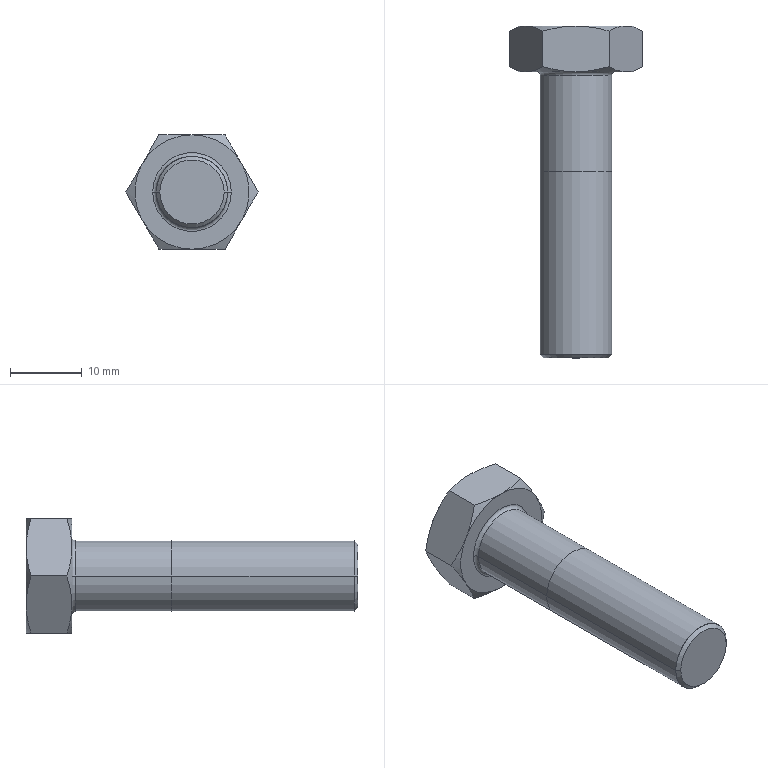Part | NX | features BREP 2 | 1 solid | 31 faces | box 18.475 x 46.4 x 16 mm | volume 5287 mm3 | cone 14 | plane 11 | cylinder 4 | torus 2 | commonest cylinder face diameters 8.376 x2 10 x2